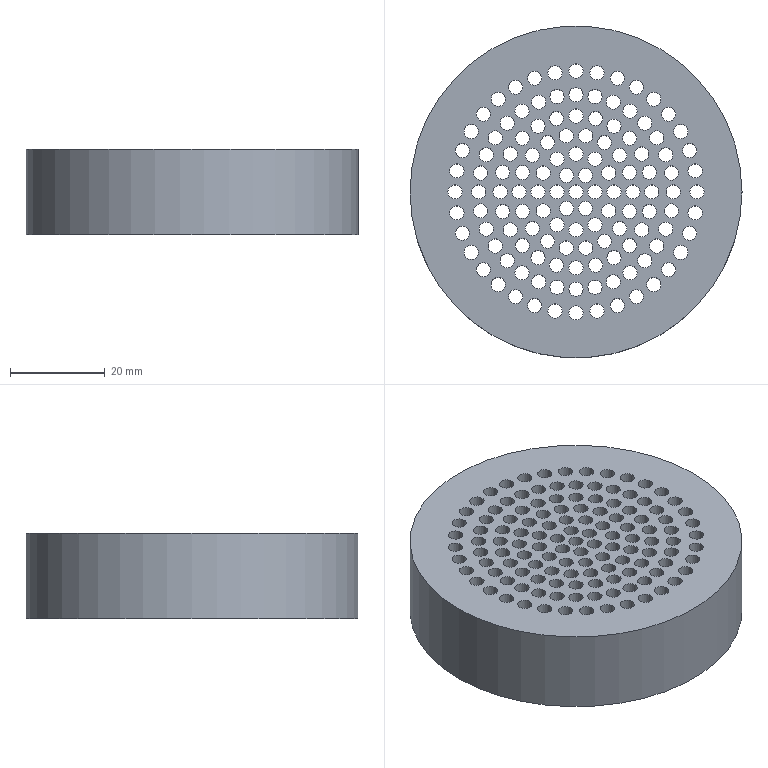NC program | NX | posted with a generic post | part box 70 x 70 x 18 mm
Whole program:
N10 G17 G21 G94 G90
(DRILLING , TOOL : ZXZ)
N12 T01 M6
N14 G54
N16 G17 G0 G90 X-3.999 Y-20.106 S3000 M3
N18 G43 Z30. H1
N20 G94 G81 G98 Z-1. F250. R3.
N22 X-7.845 Y-18.94
N24 X-11.389 Y-17.045
N26 X-14.496 Y-14.496
N28 X-17.045 Y-11.389
N30 X-18.94 Y-7.845
N32 X-20.106 Y-3.999
N34 X-20.5 Y0.
N36 X-20.106 Y3.999
N38 X-18.94 Y7.845
N40 X-17.045 Y11.389
N42 X-14.496 Y14.496
N44 X-11.389 Y17.045
N46 X-7.845 Y18.94
N48 X-3.999 Y20.106
N50 X0. Y20.5
N52 X3.999 Y20.106
N54 X7.845 Y18.94
N56 X11.389 Y17.045
N58 X14.496 Y14.496
N60 X17.045 Y11.389
N62 X18.94 Y7.845
N64 X20.106 Y3.999
N66 X20.5 Y0.
N68 X20.106 Y-3.999
N70 X18.94 Y-7.845
N72 X15.455 Y-4.141
N74 X11.276 Y-4.104
N76 X6.928 Y-4.
N78 X4. Y-6.928
N80 X2. Y-3.464
N82 X4. Y0.
N84 X8.
N86 X6.928 Y4.
N88 X9.193 Y7.713
N90 X11.276 Y4.104
N92 X12. Y0.
N94 X16.
N96 X15.455 Y4.141
N98 X13.856 Y8.
N100 X11.314 Y11.314
N102 X8. Y13.856
N104 X6. Y10.392
N106 X4. Y6.928
N108 X0. Y8.
N110 X-2.084 Y11.818
N112 X2.084
N114 X4.141 Y15.455
N116 X0. Y16.
N118 X-4.141 Y15.455
N120 X-8. Y13.856
N122 X-11.314 Y11.314
N124 X-13.856 Y8.
N126 X-15.455 Y4.141
N128 X-16. Y0.
N130 X-15.455 Y-4.141
N132 X-13.856 Y-8.
N134 X-11.314 Y-11.314
N136 X-9.193 Y-7.713
N138 X-11.276 Y-4.104
N140 X-12. Y0.
N142 X-8.
N144 X-6.928 Y4.
N146 X-11.276 Y4.104
N148 X-9.193 Y7.713
N150 X-6. Y10.392
N152 X-4. Y6.928
N154 X-2. Y3.464
N156 X2.
N158 X0. Y0.
N160 X-4.
N162 X-2. Y-3.464
N164 X-6.928 Y-4.
N166 X-4. Y-6.928
N168 X0. Y-8.
N170 X2.084 Y-11.818
N172 X-2.084
N174 X-6. Y-10.392
N176 X-8. Y-13.856
N178 X-4.141 Y-15.455
N180 X0. Y-16.
N182 X4.141 Y-15.455
N184 X8. Y-13.856
N186 X6. Y-10.392
N188 X9.193 Y-7.713
N190 X11.314 Y-11.314
N192 X13.856 Y-8.
N194 X17.045 Y-11.389
N196 X14.496 Y-14.496
N198 X11.389 Y-17.045
N200 X7.845 Y-18.94
N202 X3.999 Y-20.106
N204 X0. Y-20.5
N206 Y-25.5
N208 X-4.428 Y-25.113
N210 X-8.722 Y-23.962
N212 X-12.75 Y-22.084
N214 X-16.391 Y-19.534
N216 X-19.534 Y-16.391
N218 X-22.084 Y-12.75
N220 X-23.962 Y-8.722
N222 X-25.113 Y-4.428
N224 X-25.5 Y0.
N226 X-25.113 Y4.428
N228 X-23.962 Y8.722
N230 X-22.084 Y12.75
N232 X-19.534 Y16.391
N234 X-16.391 Y19.534
N236 X-12.75 Y22.084
N238 X-8.722 Y23.962
N240 X-4.428 Y25.113
N242 X0. Y25.5
N244 X4.428 Y25.113
N246 X8.722 Y23.962
N248 X12.75 Y22.084
N250 X16.391 Y19.534
N252 X19.534 Y16.391
N254 X22.084 Y12.75
N256 X23.962 Y8.722
N258 X25.113 Y4.428
N260 X25.5 Y0.
N262 X25.113 Y-4.428
N264 X23.962 Y-8.722
N266 X22.084 Y-12.75
N268 X19.534 Y-16.391
N270 X16.391 Y-19.534
N272 X12.75 Y-22.084
N274 X8.722 Y-23.962
N276 X4.428 Y-25.113
N278 G80
N280 G0 X4.428 Y-25.113 Z30.
N282 M5
(DRILLING_COPY , TOOL : 3.0ZT)
N284 T13 M6
N286 G54
N288 G17 G0 G90 X-3.999 Y-20.106 S2971 M3
N290 G43 Z30. H13
N292 G94 G83 G98 Z-19.901 F120. Q2. R3.
N294 X-7.845 Y-18.94
N296 X-11.389 Y-17.045
N298 X-14.496 Y-14.496
N300 X-17.045 Y-11.389
N302 X-18.94 Y-7.845
N304 X-20.106 Y-3.999
N306 X-20.5 Y0.
N308 X-20.106 Y3.999
N310 X-18.94 Y7.845
N312 X-17.045 Y11.389
N314 X-14.496 Y14.496
N316 X-11.389 Y17.045
N318 X-7.845 Y18.94
N320 X-3.999 Y20.106
N322 X0. Y20.5
N324 X3.999 Y20.106
N326 X7.845 Y18.94
N328 X11.389 Y17.045
N330 X14.496 Y14.496
N332 X17.045 Y11.389
N334 X18.94 Y7.845
N336 X20.106 Y3.999
N338 X20.5 Y0.
N340 X20.106 Y-3.999
N342 X18.94 Y-7.845
N344 X15.455 Y-4.141
N346 X11.276 Y-4.104
N348 X6.928 Y-4.
N350 X4. Y-6.928
N352 X2. Y-3.464
N354 X4. Y0.
N356 X8.
N358 X6.928 Y4.
N360 X9.193 Y7.713
N362 X11.276 Y4.104
N364 X12. Y0.
N366 X16.
N368 X15.455 Y4.141
N370 X13.856 Y8.
N372 X11.314 Y11.314
N374 X8. Y13.856
N376 X6. Y10.392
N378 X4. Y6.928
N380 X0. Y8.
N382 X-2.084 Y11.818
N384 X2.084
N386 X4.141 Y15.455
N388 X0. Y16.
N390 X-4.141 Y15.455
N392 X-8. Y13.856
N394 X-11.314 Y11.314
N396 X-13.856 Y8.
N398 X-15.455 Y4.141
N400 X-16. Y0.
N402 X-15.455 Y-4.141
N404 X-13.856 Y-8.
N406 X-11.314 Y-11.314
N408 X-9.193 Y-7.713
N410 X-11.276 Y-4.104
N412 X-12. Y0.
N414 X-8.
N416 X-6.928 Y4.
N418 X-11.276 Y4.104
N420 X-9.193 Y7.713
N422 X-6. Y10.392
N424 X-4. Y6.928
N426 X-2. Y3.464
N428 X2.
N430 X0. Y0.
N432 X-4.
N434 X-2. Y-3.464
N436 X-6.928 Y-4.
N438 X-4. Y-6.928
N440 X0. Y-8.
N442 X2.084 Y-11.818
N444 X-2.084
N446 X-6. Y-10.392
N448 X-8. Y-13.856
N450 X-4.141 Y-15.455
N452 X0. Y-16.
N454 X4.141 Y-15.455
N456 X8. Y-13.856
N458 X6. Y-10.392
N460 X9.193 Y-7.713
N462 X11.314 Y-11.314
N464 X13.856 Y-8.
N466 X17.045 Y-11.389
N468 X14.496 Y-14.496
N470 X11.389 Y-17.045
N472 X7.845 Y-18.94
N474 X3.999 Y-20.106
N476 X0. Y-20.5
N478 Y-25.5
N480 X-4.428 Y-25.113
N482 X-8.722 Y-23.962
N484 X-12.75 Y-22.084
N486 X-16.391 Y-19.534
N488 X-19.534 Y-16.391
N490 X-22.084 Y-12.75
N492 X-23.962 Y-8.722
N494 X-25.113 Y-4.428
N496 X-25.5 Y0.
N498 X-25.113 Y4.428
N500 X-23.962 Y8.722
N502 X-22.084 Y12.75
N504 X-19.534 Y16.391
N506 X-16.391 Y19.534
N508 X-12.75 Y22.084
N510 X-8.722 Y23.962
N512 X-4.428 Y25.113
N514 X0. Y25.5
N516 X4.428 Y25.113
N518 X8.722 Y23.962
N520 X12.75 Y22.084
N522 X16.391 Y19.534
N524 X19.534 Y16.391
N526 X22.084 Y12.75
N528 X23.962 Y8.722
N530 X25.113 Y4.428
N532 X25.5 Y0.
N534 X25.113 Y-4.428
N536 X23.962 Y-8.722
N538 X22.084 Y-12.75
N540 X19.534 Y-16.391
N542 X16.391 Y-19.534
N544 X12.75 Y-22.084
N546 X8.722 Y-23.962
N548 X4.428 Y-25.113
N550 G80
N552 G0 X4.428 Y-25.113 Z30.
N554 M5
(DRILLING_COPY_1 , TOOL : D6A45)
N556 T07 M6
N558 G54
N560 G17 G0 G90 X-3.999 Y-20.106 S3000 M3
N562 G43 Z30. H7
N564 G94 G81 G98 Z-1.6 F250. R3.
N566 X-7.845 Y-18.94
N568 X-11.389 Y-17.045
N570 X-14.496 Y-14.496
N572 X-17.045 Y-11.389
N574 X-18.94 Y-7.845
N576 X-20.106 Y-3.999
N578 X-20.5 Y0.
N580 X-20.106 Y3.999
N582 X-18.94 Y7.845
N584 X-17.045 Y11.389
N586 X-14.496 Y14.496
N588 X-11.389 Y17.045
N590 X-7.845 Y18.94
N592 X-3.999 Y20.106
N594 X0. Y20.5
N596 X3.999 Y20.106
N598 X7.845 Y18.94
N600 X11.389 Y17.045
N602 X14.496 Y14.496
N604 X17.045 Y11.389
N606 X18.94 Y7.845
N608 X20.106 Y3.999
N610 X20.5 Y0.
N612 X20.106 Y-3.999
N614 X18.94 Y-7.845
N616 X15.455 Y-4.141
N618 X11.276 Y-4.104
N620 X6.928 Y-4.
N622 X4. Y-6.928
N624 X2. Y-3.464
N626 X4. Y0.
N628 X8.
N630 X6.928 Y4.
N632 X9.193 Y7.713
N634 X11.276 Y4.104
N636 X12. Y0.
N638 X16.
N640 X15.455 Y4.141
N642 X13.856 Y8.
N644 X11.314 Y11.314
N646 X8. Y13.856
N648 X6. Y10.392
N650 X4. Y6.928
N652 X0. Y8.
N654 X-2.084 Y11.818
N656 X2.084
N658 X4.141 Y15.455
N660 X0. Y16.
N662 X-4.141 Y15.455
N664 X-8. Y13.856
N666 X-11.314 Y11.314
N668 X-13.856 Y8.
N670 X-15.455 Y4.141
N672 X-16. Y0.
N674 X-15.455 Y-4.141
N676 X-13.856 Y-8.
N678 X-11.314 Y-11.314
N680 X-9.193 Y-7.713
N682 X-11.276 Y-4.104
N684 X-12. Y0.
N686 X-8.
N688 X-6.928 Y4.
N690 X-11.276 Y4.104
N692 X-9.193 Y7.713
N694 X-6. Y10.392
N696 X-4. Y6.928
N698 X-2. Y3.464
N700 X2.
N702 X0. Y0.
N704 X-4.
N706 X-2. Y-3.464
N708 X-6.928 Y-4.
N710 X-4. Y-6.928
N712 X0. Y-8.
N714 X2.084 Y-11.818
N716 X-2.084
N718 X-6. Y-10.392
N720 X-8. Y-13.856
N722 X-4.141 Y-15.455
N724 X0. Y-16.
N726 X4.141 Y-15.455
N728 X8. Y-13.856
N730 X6. Y-10.392
N732 X9.193 Y-7.713
N734 X11.314 Y-11.314
N736 X13.856 Y-8.
N738 X17.045 Y-11.389
N740 X14.496 Y-14.496
N742 X11.389 Y-17.045
N744 X7.845 Y-18.94
N746 X3.999 Y-20.106
N748 X0. Y-20.5
N750 Y-25.5
N752 X-4.428 Y-25.113
N754 X-8.722 Y-23.962
N756 X-12.75 Y-22.084
N758 X-16.391 Y-19.534
N760 X-19.534 Y-16.391
N762 X-22.084 Y-12.75
N764 X-23.962 Y-8.722
N766 X-25.113 Y-4.428
N768 X-25.5 Y0.
N770 X-25.113 Y4.428
N772 X-23.962 Y8.722
N774 X-22.084 Y12.75
N776 X-19.534 Y16.391
N778 X-16.391 Y19.534
N780 X-12.75 Y22.084
N782 X-8.722 Y23.962
N784 X-4.428 Y25.113
N786 X0. Y25.5
N788 X4.428 Y25.113
N790 X8.722 Y23.962
N792 X12.75 Y22.084
N794 X16.391 Y19.534
N796 X19.534 Y16.391
N798 X22.084 Y12.75
N800 X23.962 Y8.722
N802 X25.113 Y4.428
N804 X25.5 Y0.
N806 X25.113 Y-4.428
N808 X23.962 Y-8.722
N810 X22.084 Y-12.75
N812 X19.534 Y-16.391
N814 X16.391 Y-19.534
N816 X12.75 Y-22.084
N818 X8.722 Y-23.962
N820 X4.428 Y-25.113
N822 G80
N824 G0 X4.428 Y-25.113 Z30.
N826 M5
N828 M2